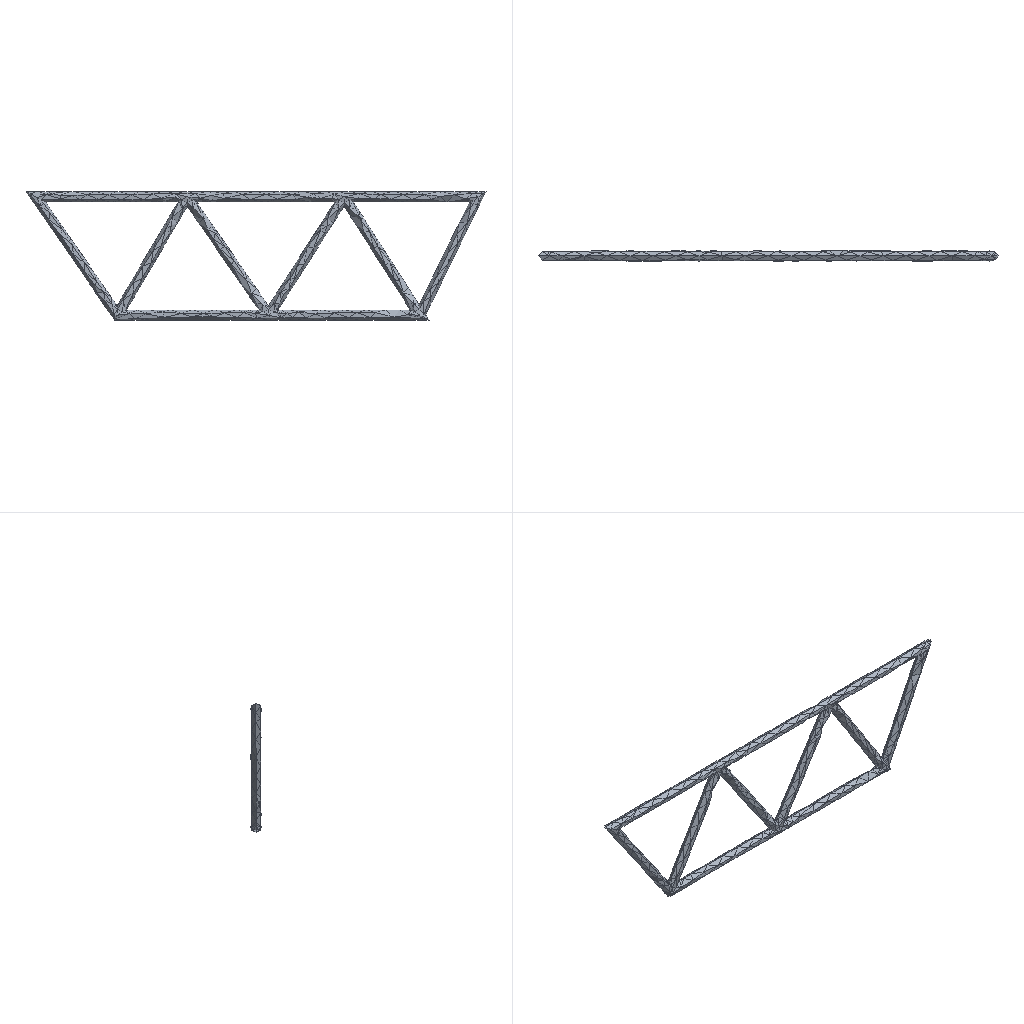Simulation study | ansys workbench
Ansys APDL input file, long lists of numbers shortened:
/batch
/config,noeldb,1     ! force off writing results to database
*get,_wallstrt,active,,time,wall
! ANSYS input file written by Workbench version 2022 R1
! File used for geometry attach: F:\ansys（分析文件汇总)\桥梁分析\桥梁_files\dp0\SYS-1\DM\SYS-1.scdoc
/title,__--____ (B5)
! ****** Begin Custom Load Command Snippet ******
/COM, ACT Extensions:
/COM,     LSDYNA, 2021.1
/COM,
! ****** End   Custom Load Command Snippet ******
*DIM,_wb_ProjectScratch_dir,string,248
_wb_ProjectScratch_dir(1) = 'F:\ansys（分析文件汇总)\桥梁分析\_ProjectScratch\ScrE515\'
*DIM,_wb_SolverFiles_dir,string,248
_wb_SolverFiles_dir(1) = 'F:\ansys（分析文件汇总)\桥梁分析\桥梁_files\dp0\SYS-1\MECH\'
*DIM,_wb_userfiles_dir,string,248
_wb_userfiles_dir(1) = 'F:\ansys（分析文件汇总)\桥梁分析\桥梁_files\user_files\'
/com,--- Data in consistent NMM units. See Solving Units in the help system for more information.
/units,MPA
/nopr
/wb,file,start              !  signify a WB generated input file
/prep7
! Turn off shape checking because checks already performed inside WB mesher.
! See help system for more information.
SHPP,OFF,,NOWARN
/nolist
etcon,set             ! allow ANSYS to choose best KEYOP's for 180x elements, resets any applicable keyopt to MAPDL defaults
/com,*********** Nodes for the whole assembly ***********
nblock,3,,108
(1i9,3e20.9e3)
        1    -6.120000000E+00     1.000000000E+00     3.044718724E+00
! (98 more lines like these left out)
-1
/wb,elem,start            !  set before creation of elements
/com,*********** Elements for Body 1 "SYS-1\Beam (_____1)" ***********
et,1,188
keyo,1,3,2
eblock,19,solid,,14
(19i9)
        1        1        1        1        0        0        0        0        3        0       15       30       32       45
! (13 more lines like these left out)
-1
/com,*********** Elements for Body 2 "SYS-1\Beam (_____1)" ***********
et,2,188
keyo,2,3,2
eblock,19,solid,,20
(19i9)
        2        2        2        2        0        0        0        0        3        0       29       59       61       80
! (19 more lines like these left out)
-1
/com,*********** Elements for Body 3 "SYS-1\Beam (_____1)" ***********
et,3,188
keyo,3,3,2
eblock,19,solid,,14
(19i9)
        3        3        3        3        0        0        0        0        3        0        1        1        3       16
! (13 more lines like these left out)
-1
/wb,elem,end               !  done creating elements
/com,*********** Send User Defined Coordinate System(s) ***********
csys,0
toffst,273.15,  ! Temperature offset from absolute zero
/com,*********** Set Reference Temperature ***********
tref,22.
/wb,mat,start              !  starting to send materials
/com,*********** Send Materials ***********
Temperature = 'TEMP' ! Temperature
MP,DENS,1,7.85e-09,	! tonne mm^-3
MP,ALPX,1,1.2e-05,	! C^-1
MP,C,1,434000000,	! mm^2 s^-2 C^-1
MP,KXX,1,60.5,	! tonne mm s^-3 C^-1
MP,RSVX,1,0.00017,	! ohm mm
MP,EX,1,200000,	! tonne s^-2 mm^-1
MP,NUXY,1,0.3,
MP,MURX,1,10000,
Temperature = 'TEMP' ! Temperature
MP,DENS,2,7.85e-09,	! tonne mm^-3
MP,ALPX,2,1.2e-05,	! C^-1
MP,C,2,434000000,	! mm^2 s^-2 C^-1
MP,KXX,2,60.5,	! tonne mm s^-3 C^-1
MP,RSVX,2,0.00017,	! ohm mm
MP,EX,2,200000,	! tonne s^-2 mm^-1
MP,NUXY,2,0.3,
MP,MURX,2,10000,
Temperature = 'TEMP' ! Temperature
MP,DENS,3,7.85e-09,	! tonne mm^-3
MP,ALPX,3,1.2e-05,	! C^-1
MP,C,3,434000000,	! mm^2 s^-2 C^-1
MP,KXX,3,60.5,	! tonne mm s^-3 C^-1
MP,RSVX,3,0.00017,	! ohm mm
MP,EX,3,200000,	! tonne s^-2 mm^-1
MP,NUXY,3,0.3,
MP,MURX,3,10000,
/wb,mat,end                !  done sending materials
/com,*********** Send Beam Properties ***********
SECTYPE,1,BEAM,RECT
SECDATA,0.2,2.
secoffset,cent
SECTYPE,2,BEAM,RECT
SECDATA,0.2,2.
secoffset,cent
SECTYPE,3,BEAM,RECT
SECDATA,0.2,2.
secoffset,cent
!************************* Model Summary ********************
!SYS-1\Beam (_____1),	结构钢,	matid,	1
!SYS-1\Beam (_____1),	结构钢,	matid,	2
!SYS-1\Beam (_____1),	结构钢,	matid,	3
!************************* End Model Summary ********************
! get the diagonal of the bounding box. Needed later for other things
*get,_xmin,node,,mnloc,x
*get,_ymin,node,,mnloc,y
*get,_zmin,node,,mnloc,z
*get,_xmax,node,,mxloc,x
*get,_ymax,node,,mxloc,y
*get,_zmax,node,,mxloc,z
_ASMDIAG=(_xmax-_xmin)*(_xmax-_xmin)+(_ymax-_ymin)*(_ymax-_ymin)+(_zmax-_zmin)*(_zmax-_zmin)
_ASMDIAG=SQRT(_ASMDIAG)
/wb,contact,start          !  starting to send contact
/wb,contact,end            !  done creating contacts
/golist
/wb,load,start             !  starting to send loads
/com,*********** Fixed Supports ***********
CMBLOCK,_FIXEDSU,NODE,        3
(8i10)
         1        30        59
cmsel,s,_FIXEDSU
d,all,all
nsel,all
/com,*********** Define Force Using Surface Effect Elements ***********
local,12,0,0.,0.,0.,0.,0.,0.
csys,0
et,4,156
keyop,4,5,1         !  No orientation node
eblock,10,,,20
(15i9)
       49        4        4        4       12       59       61
! (19 more lines like these left out)
-1
esel,s,type,,4
keyop,4,2,1                ! Apply load in local coordinate system
keyop,4,7,1                ! Use original area so load is constant in large deformation
esel,all
/gst,on,on
fini
*get,_numnode,node,0,count
*get,_numelem,elem,0,count
*get, _MAXELEMNUM, elem, 0, NUM, MAX
*get, _MAXNODENUM, node, 0, NUM, MAX
*get, _MAXELEMTYPE, etyp, 0, NUM, MAX
*get, _MAXREALCONST, real, 0, NUM, MAX
/go
/wb,load,end               !  done creating loads
/com,--- Number of total nodes = %_numnode%
/com,--- Number of contact elements = 20
/com,--- Number of spring elements = 0
/com,--- Number of bearing elements = 0
/com,--- Number of solid elements = 48
/com,--- Number of condensed parts = 0
/com,--- Number of total elements = %_numelem%
*get,_wallbsol,active,,time,wall
/com,****************************************************************************
/com,*************************    SOLUTION       ********************************
/com,****************************************************************************
/solu
antype,0                   ! static analysis
_thickRatio=  0     ! Ratio of thick parts in the model
eqsl,sparse,,,,,1
cntr,print,1               ! print out contact info and also make no initial contact an error
dmpoption,emat,no             ! Don't combine emat file for DANSYS
dmpoption,esav,no             ! Don't combine esav file for DANSYS
nldiag,cont,iter           ! print out contact info each equilibrium iteration
rescontrol,,none                 ! Do not keep any restart files
/com,****************************************************
/com,******************* SOLVE FOR LS 1 OF 1 ****************
esel,s,type,,4
nsle
sfe,all,1,pres,1,0.
sfe,all,2,pres,1,0.
sfe,all,3,pres,1,7.512
nsel,all
esel,all
/nopr
/gopr
nsub,1,1,1
time,1.
outres,erase
outres,all,none
outres,nsol,all,
outres,rsol,all
outres,eangl,all
outres,etmp,all
outres,veng,all
outres,strs,all,
outres,epel,all,
outres,eppl,all,
outres,cont,all,
/nopr
esel,s,type,,1
esel,a,type,,2,3
cm,_elmisc,elem
esel,all
/gopr
outres,misc,all,_elmisc
! *********** WB SOLVE COMMAND ***********
! check interactive state
*get,ANSINTER_,active,,int
*if,ANSINTER_,ne,0,then
/eof
*endif
solve
/com *************** Write FE CONNECTORS *********
CEWRITE,file,ce,,INTE
/com,****************************************************
/com,*************** FINISHED SOLVE FOR LS 1 *************
*get,_wallasol,active,,time,wall
/nopr
*get,_numnode,node,0,count
*get,_numelem,elem,0,count
*get, _MAXELEMNUM, elem, 0, NUM, MAX
*get, _MAXNODENUM, node, 0, NUM, MAX,,,INTERNAL
*get, _MAXELEMTYPE, etyp, 0, NUM, MAX
*get, _MAXREALCONST, real, 0, NUM, MAX
/gopr
/post1
xmlo,ENCODING,ISO-8859-1
xmlo,parm
/xml,parm,xml
fini
/gopr
*get,_walldone,active,,time,wall
_preptime=(_wallbsol-_wallstrt)*3600
_solvtime=(_wallasol-_wallbsol)*3600
_posttime=(_walldone-_wallasol)*3600
_totaltim=(_walldone-_wallstrt)*3600
*get,_dlbratio,active,0,solu,dlbr
*get,_combtime,active,0,solu,comb
*get,_ssmode,active,0,solu,ssmm
*get,_ndofs,active,0,solu,ndof
*get,_sol_end_time,active,0,set,time
*if,_sol_end_time,eq,1.,then
/fclean				!clean distributed files
*endif
/com,--- Total number of nodes = %_numnode%
/com,--- Total number of elements = %_numelem%
/com,--- Element load balance ratio = %_dlbratio%
/com,--- Time to combine distributed files = %_combtime%
/com,--- Sparse memory mode = %_ssmode%
/com,--- Number of DOF = %_ndofs%
/wb,file,end               ! done with WB generated input